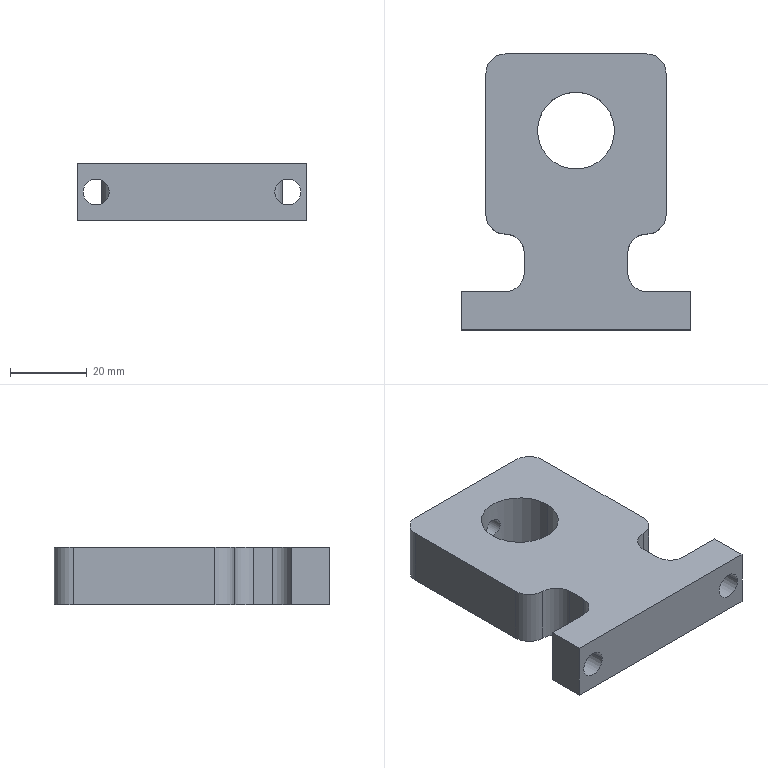Part | SolidWorks | features ICE 3, CirPattern 1, Extrusion 1, Fillet 1, HoleWzd 1 | 1 solid | 28 faces | box 60 x 72 x 15 mm | volume 42527 mm3 | cylinder 16 | plane 12 | commonest cylinder face diameters 10 x8 6.8 x4 5 x2 20.1 x2
STEP:
#1=CARTESIAN_POINT('',(0.,62.05,-2.5));
#2=VERTEX_POINT('',#1);
#3=CARTESIAN_POINT('',(0.,62.05,2.5));
#4=VERTEX_POINT('',#3);
#5=CARTESIAN_POINT('',(0.,62.05,-2.5));
#6=CARTESIAN_POINT('',(-0.327,62.05,-2.5));
#7=CARTESIAN_POINT('',(-0.6572,62.033,-2.434));
#8=CARTESIAN_POINT('',(-1.109,61.99,-2.247));
#9=CARTESIAN_POINT('',(-1.255,61.972,-2.168));
#10=CARTESIAN_POINT('',(-1.526,61.934,-1.987));
#11=CARTESIAN_POINT('',(-1.652,61.914,-1.884));
#12=CARTESIAN_POINT('',(-1.882,61.873,-1.653));
#13=CARTESIAN_POINT('',(-1.987,61.852,-1.525));
#14=CARTESIAN_POINT('',(-2.168,61.814,-1.255));
#15=CARTESIAN_POINT('',(-2.245,61.796,-1.112));
#16=CARTESIAN_POINT('',(-2.372,61.766,-0.808));
#17=CARTESIAN_POINT('',(-2.419,61.755,-0.6506));
#18=CARTESIAN_POINT('',(-2.483,61.738,-0.3307));
#19=CARTESIAN_POINT('',(-2.5,61.734,-0.1657));
#20=CARTESIAN_POINT('',(-2.5,61.734,0.1641));
#21=CARTESIAN_POINT('',(-2.484,61.738,0.3268));
#22=CARTESIAN_POINT('',(-2.42,61.754,0.6479));
#23=CARTESIAN_POINT('',(-2.372,61.766,0.8074));
#24=CARTESIAN_POINT('',(-2.247,61.796,1.109));
#25=CARTESIAN_POINT('',(-2.17,61.813,1.252));
#26=CARTESIAN_POINT('',(-1.988,61.852,1.525));
#27=CARTESIAN_POINT('',(-1.883,61.873,1.652));
#28=CARTESIAN_POINT('',(-1.654,61.914,1.882));
#29=CARTESIAN_POINT('',(-1.527,61.934,1.986));
#30=CARTESIAN_POINT('',(-1.255,61.972,2.168));
#31=CARTESIAN_POINT('',(-1.112,61.989,2.245));
#32=CARTESIAN_POINT('',(-0.8107,62.018,2.371));
#33=CARTESIAN_POINT('',(-0.6515,62.03,2.419));
#34=CARTESIAN_POINT('',(-0.3293,62.046,2.484));
#35=CARTESIAN_POINT('',(-0.1658,62.05,2.5));
#36=CARTESIAN_POINT('',(0.,62.05,2.5));
#37=B_SPLINE_CURVE_WITH_KNOTS('',3,(#5,#6,#7,#8,#9,#10,#11,#12,#13,#14,#15,#16,#17,#18,#19,#20,#21,#22,#23,#24,#25,#26,#27,#28,#29,#30,#31,#32,#33,#34,#35,#36),.UNSPECIFIED.,.F.,.F.,(4,2,2,2,2,2,2,2,2,2,2,2,2,2,2,4),(0.007847,0.008828,0.009318,0.009808,0.0103,0.01079,0.01128,0.01177,0.01226,0.01275,0.01324,0.01373,0.01422,0.01471,0.0152,0.01569),.UNSPECIFIED.);
#38=EDGE_CURVE('',#2,#4,#37,.T.);
#39=ORIENTED_EDGE('',*,*,#38,.F.);
#40=CARTESIAN_POINT('',(0.,72.,-2.5));
#41=VERTEX_POINT('',#40);
#42=CARTESIAN_POINT('',(0.,72.,-2.5));
#43=DIRECTION('',(0.,1.,0.));
#44=VECTOR('',#43,1000.);
#45=LINE('',#42,#44);
#46=EDGE_CURVE('',#2,#41,#45,.T.);
#47=ORIENTED_EDGE('',*,*,#46,.T.);
#48=CARTESIAN_POINT('',(0.,72.,2.5));
#49=VERTEX_POINT('',#48);
#50=CARTESIAN_POINT('',(0.,72.,0.));
#51=DIRECTION('',(0.,1.,0.));
#52=DIRECTION('',(0.,0.,1.));
#53=AXIS2_PLACEMENT_3D('',#50,#51,#52);
#54=CIRCLE('',#53,2.5);
#55=EDGE_CURVE('',#41,#49,#54,.T.);
#56=ORIENTED_EDGE('',*,*,#55,.T.);
#57=CARTESIAN_POINT('',(0.,72.,2.5));
#58=DIRECTION('',(0.,1.,0.));
#59=VECTOR('',#58,1000.);
#60=LINE('',#57,#59);
#61=EDGE_CURVE('',#4,#49,#60,.T.);
#62=ORIENTED_EDGE('',*,*,#61,.F.);
#63=EDGE_LOOP('',(#39,#47,#56,#62));
#64=FACE_OUTER_BOUND('',#63,.T.);
#65=CARTESIAN_POINT('',(0.,72.,0.));
#66=DIRECTION('',(0.,1.,0.));
#67=DIRECTION('',(0.,0.,1.));
#68=AXIS2_PLACEMENT_3D('',#65,#66,#67);
#69=CYLINDRICAL_SURFACE('',#68,2.5);
#70=ADVANCED_FACE('',(#64),#69,.F.);
#71=CARTESIAN_POINT('',(-21.6,10.,0.));
#72=VERTEX_POINT('',#71);
#73=CARTESIAN_POINT('',(-28.4,10.,0.));
#74=VERTEX_POINT('',#73);
#75=CARTESIAN_POINT('',(-25.,10.,0.));
#76=DIRECTION('',(0.,1.,0.));
#77=DIRECTION('',(1.,0.,0.));
#78=AXIS2_PLACEMENT_3D('',#75,#76,#77);
#79=CIRCLE('',#78,3.4);
#80=EDGE_CURVE('',#72,#74,#79,.T.);
#81=ORIENTED_EDGE('',*,*,#80,.T.);
#82=CARTESIAN_POINT('',(-28.4,0.,0.));
#83=VERTEX_POINT('',#82);
#84=CARTESIAN_POINT('',(-28.4,72.001,0.));
#85=DIRECTION('',(0.,-1.,0.));
#86=VECTOR('',#85,1000.);
#87=LINE('',#84,#86);
#88=EDGE_CURVE('',#74,#83,#87,.T.);
#89=ORIENTED_EDGE('',*,*,#88,.T.);
#90=CARTESIAN_POINT('',(-21.6,0.,0.));
#91=VERTEX_POINT('',#90);
#92=CARTESIAN_POINT('',(-25.,0.,0.));
#93=DIRECTION('',(0.,-1.,0.));
#94=DIRECTION('',(1.,0.,0.));
#95=AXIS2_PLACEMENT_3D('',#92,#93,#94);
#96=CIRCLE('',#95,3.4);
#97=EDGE_CURVE('',#83,#91,#96,.T.);
#98=ORIENTED_EDGE('',*,*,#97,.T.);
#99=CARTESIAN_POINT('',(-21.6,72.001,0.));
#100=DIRECTION('',(0.,-1.,0.));
#101=VECTOR('',#100,1000.);
#102=LINE('',#99,#101);
#103=EDGE_CURVE('',#72,#91,#102,.T.);
#104=ORIENTED_EDGE('',*,*,#103,.F.);
#105=EDGE_LOOP('',(#81,#89,#98,#104));
#106=FACE_OUTER_BOUND('',#105,.T.);
#107=CARTESIAN_POINT('',(-25.,72.001,0.));
#108=DIRECTION('',(0.,-1.,0.));
#109=DIRECTION('',(1.,0.,0.));
#110=AXIS2_PLACEMENT_3D('',#107,#108,#109);
#111=CYLINDRICAL_SURFACE('',#110,3.4);
#112=ADVANCED_FACE('',(#106),#111,.F.);
#113=CARTESIAN_POINT('',(28.4,10.,0.));
#114=VERTEX_POINT('',#113);
#115=CARTESIAN_POINT('',(21.6,10.,0.));
#116=VERTEX_POINT('',#115);
#117=CARTESIAN_POINT('',(25.,10.,0.));
#118=DIRECTION('',(0.,1.,0.));
#119=DIRECTION('',(1.,0.,0.));
#120=AXIS2_PLACEMENT_3D('',#117,#118,#119);
#121=CIRCLE('',#120,3.4);
#122=EDGE_CURVE('',#114,#116,#121,.T.);
#123=ORIENTED_EDGE('',*,*,#122,.T.);
#124=CARTESIAN_POINT('',(21.6,0.,0.));
#125=VERTEX_POINT('',#124);
#126=CARTESIAN_POINT('',(21.6,72.001,0.));
#127=DIRECTION('',(0.,-1.,0.));
#128=VECTOR('',#127,1000.);
#129=LINE('',#126,#128);
#130=EDGE_CURVE('',#116,#125,#129,.T.);
#131=ORIENTED_EDGE('',*,*,#130,.T.);
#132=CARTESIAN_POINT('',(28.4,0.,0.));
#133=VERTEX_POINT('',#132);
#134=CARTESIAN_POINT('',(25.,0.,0.));
#135=DIRECTION('',(0.,-1.,0.));
#136=DIRECTION('',(-1.,0.,0.));
#137=AXIS2_PLACEMENT_3D('',#134,#135,#136);
#138=CIRCLE('',#137,3.4);
#139=EDGE_CURVE('',#125,#133,#138,.T.);
#140=ORIENTED_EDGE('',*,*,#139,.T.);
#141=CARTESIAN_POINT('',(28.4,72.001,0.));
#142=DIRECTION('',(0.,-1.,0.));
#143=VECTOR('',#142,1000.);
#144=LINE('',#141,#143);
#145=EDGE_CURVE('',#114,#133,#144,.T.);
#146=ORIENTED_EDGE('',*,*,#145,.F.);
#147=EDGE_LOOP('',(#123,#131,#140,#146));
#148=FACE_OUTER_BOUND('',#147,.T.);
#149=CARTESIAN_POINT('',(25.,72.001,0.));
#150=DIRECTION('',(0.,-1.,0.));
#151=DIRECTION('',(1.,0.,0.));
#152=AXIS2_PLACEMENT_3D('',#149,#150,#151);
#153=CYLINDRICAL_SURFACE('',#152,3.4);
#154=ADVANCED_FACE('',(#148),#153,.F.);
#155=CARTESIAN_POINT('',(-10.05,52.,-7.5));
#156=VERTEX_POINT('',#155);
#157=CARTESIAN_POINT('',(10.05,52.,-7.5));
#158=VERTEX_POINT('',#157);
#159=CARTESIAN_POINT('',(0.,52.,-7.5));
#160=DIRECTION('',(0.,0.,1.));
#161=DIRECTION('',(1.,0.,0.));
#162=AXIS2_PLACEMENT_3D('',#159,#160,#161);
#163=CIRCLE('',#162,10.05);
#164=EDGE_CURVE('',#156,#158,#163,.T.);
#165=ORIENTED_EDGE('',*,*,#164,.F.);
#166=CARTESIAN_POINT('',(-10.05,52.,7.5));
#167=VERTEX_POINT('',#166);
#168=CARTESIAN_POINT('',(-10.05,52.,-7.5));
#169=DIRECTION('',(0.,0.,1.));
#170=VECTOR('',#169,1000.);
#171=LINE('',#168,#170);
#172=EDGE_CURVE('',#156,#167,#171,.T.);
#173=ORIENTED_EDGE('',*,*,#172,.T.);
#174=CARTESIAN_POINT('',(10.05,52.,7.5));
#175=VERTEX_POINT('',#174);
#176=CARTESIAN_POINT('',(0.,52.,7.5));
#177=DIRECTION('',(0.,0.,1.));
#178=DIRECTION('',(1.,0.,0.));
#179=AXIS2_PLACEMENT_3D('',#176,#177,#178);
#180=CIRCLE('',#179,10.05);
#181=EDGE_CURVE('',#167,#175,#180,.T.);
#182=ORIENTED_EDGE('',*,*,#181,.T.);
#183=CARTESIAN_POINT('',(10.05,52.,-7.5));
#184=DIRECTION('',(0.,0.,1.));
#185=VECTOR('',#184,1000.);
#186=LINE('',#183,#185);
#187=EDGE_CURVE('',#158,#175,#186,.T.);
#188=ORIENTED_EDGE('',*,*,#187,.F.);
#189=EDGE_LOOP('',(#165,#173,#182,#188));
#190=FACE_OUTER_BOUND('',#189,.T.);
#191=CARTESIAN_POINT('',(0.,52.,-7.5));
#192=DIRECTION('',(0.,0.,1.));
#193=DIRECTION('',(1.,0.,0.));
#194=AXIS2_PLACEMENT_3D('',#191,#192,#193);
#195=CYLINDRICAL_SURFACE('',#194,10.05);
#196=ADVANCED_FACE('',(#190),#195,.F.);
#197=CARTESIAN_POINT('',(23.5,30.,-7.5));
#198=VERTEX_POINT('',#197);
#199=CARTESIAN_POINT('',(23.5,67.,-7.5));
#200=VERTEX_POINT('',#199);
#201=CARTESIAN_POINT('',(23.5,25.,-7.5));
#202=DIRECTION('',(0.,1.,0.));
#203=VECTOR('',#202,1000.);
#204=LINE('',#201,#203);
#205=EDGE_CURVE('',#198,#200,#204,.T.);
#206=ORIENTED_EDGE('',*,*,#205,.T.);
#207=CARTESIAN_POINT('',(23.5,67.,7.5));
#208=VERTEX_POINT('',#207);
#209=CARTESIAN_POINT('',(23.5,67.,7.5));
#210=DIRECTION('',(0.,0.,1.));
#211=VECTOR('',#210,1000.);
#212=LINE('',#209,#211);
#213=EDGE_CURVE('',#200,#208,#212,.T.);
#214=ORIENTED_EDGE('',*,*,#213,.T.);
#215=CARTESIAN_POINT('',(23.5,30.,7.5));
#216=VERTEX_POINT('',#215);
#217=CARTESIAN_POINT('',(23.5,25.,7.5));
#218=DIRECTION('',(0.,1.,0.));
#219=VECTOR('',#218,1000.);
#220=LINE('',#217,#219);
#221=EDGE_CURVE('',#216,#208,#220,.T.);
#222=ORIENTED_EDGE('',*,*,#221,.F.);
#223=CARTESIAN_POINT('',(23.5,30.,7.5));
#224=DIRECTION('',(0.,0.,-1.));
#225=VECTOR('',#224,1000.);
#226=LINE('',#223,#225);
#227=EDGE_CURVE('',#216,#198,#226,.T.);
#228=ORIENTED_EDGE('',*,*,#227,.T.);
#229=EDGE_LOOP('',(#206,#214,#222,#228));
#230=FACE_OUTER_BOUND('',#229,.T.);
#231=CARTESIAN_POINT('',(23.5,25.,7.5));
#232=DIRECTION('',(-1.,0.,0.));
#233=DIRECTION('',(0.,-1.,0.));
#234=AXIS2_PLACEMENT_3D('',#231,#232,#233);
#235=PLANE('',#234);
#236=ADVANCED_FACE('',(#230),#235,.F.);
#237=CARTESIAN_POINT('',(0.,72.,0.));
#238=DIRECTION('',(0.,1.,0.));
#239=DIRECTION('',(0.,0.,1.));
#240=AXIS2_PLACEMENT_3D('',#237,#238,#239);
#241=CIRCLE('',#240,2.5);
#242=EDGE_CURVE('',#49,#41,#241,.T.);
#243=ORIENTED_EDGE('',*,*,#242,.F.);
#244=ORIENTED_EDGE('',*,*,#55,.F.);
#245=EDGE_LOOP('',(#243,#244));
#246=FACE_BOUND('',#245,.T.);
#247=CARTESIAN_POINT('',(18.5,72.,7.5));
#248=VERTEX_POINT('',#247);
#249=CARTESIAN_POINT('',(-18.5,72.,7.5));
#250=VERTEX_POINT('',#249);
#251=CARTESIAN_POINT('',(-23.5,72.,7.5));
#252=DIRECTION('',(-1.,0.,0.));
#253=VECTOR('',#252,1000.);
#254=LINE('',#251,#253);
#255=EDGE_CURVE('',#248,#250,#254,.T.);
#256=ORIENTED_EDGE('',*,*,#255,.F.);
#257=CARTESIAN_POINT('',(18.5,72.,-7.5));
#258=VERTEX_POINT('',#257);
#259=CARTESIAN_POINT('',(18.5,72.,7.5));
#260=DIRECTION('',(0.,0.,-1.));
#261=VECTOR('',#260,1000.);
#262=LINE('',#259,#261);
#263=EDGE_CURVE('',#248,#258,#262,.T.);
#264=ORIENTED_EDGE('',*,*,#263,.T.);
#265=CARTESIAN_POINT('',(-18.5,72.,-7.5));
#266=VERTEX_POINT('',#265);
#267=CARTESIAN_POINT('',(-23.5,72.,-7.5));
#268=DIRECTION('',(-1.,0.,0.));
#269=VECTOR('',#268,1000.);
#270=LINE('',#267,#269);
#271=EDGE_CURVE('',#258,#266,#270,.T.);
#272=ORIENTED_EDGE('',*,*,#271,.T.);
#273=CARTESIAN_POINT('',(-18.5,72.,7.5));
#274=DIRECTION('',(0.,0.,1.));
#275=VECTOR('',#274,1000.);
#276=LINE('',#273,#275);
#277=EDGE_CURVE('',#266,#250,#276,.T.);
#278=ORIENTED_EDGE('',*,*,#277,.T.);
#279=EDGE_LOOP('',(#256,#264,#272,#278));
#280=FACE_OUTER_BOUND('',#279,.T.);
#281=CARTESIAN_POINT('',(-23.5,72.,7.5));
#282=DIRECTION('',(0.,-1.,0.));
#283=DIRECTION('',(0.,0.,-1.));
#284=AXIS2_PLACEMENT_3D('',#281,#282,#283);
#285=PLANE('',#284);
#286=ADVANCED_FACE('',(#246,#280),#285,.F.);
#287=CARTESIAN_POINT('',(-23.5,67.,7.5));
#288=VERTEX_POINT('',#287);
#289=CARTESIAN_POINT('',(-23.5,30.,7.5));
#290=VERTEX_POINT('',#289);
#291=CARTESIAN_POINT('',(-23.5,25.,7.5));
#292=DIRECTION('',(0.,-1.,0.));
#293=VECTOR('',#292,1000.);
#294=LINE('',#291,#293);
#295=EDGE_CURVE('',#288,#290,#294,.T.);
#296=ORIENTED_EDGE('',*,*,#295,.F.);
#297=CARTESIAN_POINT('',(-23.5,67.,-7.5));
#298=VERTEX_POINT('',#297);
#299=CARTESIAN_POINT('',(-23.5,67.,7.5));
#300=DIRECTION('',(0.,0.,-1.));
#301=VECTOR('',#300,1000.);
#302=LINE('',#299,#301);
#303=EDGE_CURVE('',#288,#298,#302,.T.);
#304=ORIENTED_EDGE('',*,*,#303,.T.);
#305=CARTESIAN_POINT('',(-23.5,30.,-7.5));
#306=VERTEX_POINT('',#305);
#307=CARTESIAN_POINT('',(-23.5,25.,-7.5));
#308=DIRECTION('',(0.,-1.,0.));
#309=VECTOR('',#308,1000.);
#310=LINE('',#307,#309);
#311=EDGE_CURVE('',#298,#306,#310,.T.);
#312=ORIENTED_EDGE('',*,*,#311,.T.);
#313=CARTESIAN_POINT('',(-23.5,30.,7.5));
#314=DIRECTION('',(0.,0.,1.));
#315=VECTOR('',#314,1000.);
#316=LINE('',#313,#315);
#317=EDGE_CURVE('',#306,#290,#316,.T.);
#318=ORIENTED_EDGE('',*,*,#317,.T.);
#319=EDGE_LOOP('',(#296,#304,#312,#318));
#320=FACE_OUTER_BOUND('',#319,.T.);
#321=CARTESIAN_POINT('',(-23.5,25.,7.5));
#322=DIRECTION('',(1.,0.,0.));
#323=DIRECTION('',(0.,1.,0.));
#324=AXIS2_PLACEMENT_3D('',#321,#322,#323);
#325=PLANE('',#324);
#326=ADVANCED_FACE('',(#320),#325,.F.);
#327=CARTESIAN_POINT('',(-13.5,20.,-7.5));
#328=VERTEX_POINT('',#327);
#329=CARTESIAN_POINT('',(-13.5,15.,-7.5));
#330=VERTEX_POINT('',#329);
#331=CARTESIAN_POINT('',(-13.5,10.,-7.5));
#332=DIRECTION('',(0.,-1.,0.));
#333=VECTOR('',#332,1000.);
#334=LINE('',#331,#333);
#335=EDGE_CURVE('',#328,#330,#334,.T.);
#336=ORIENTED_EDGE('',*,*,#335,.T.);
#337=CARTESIAN_POINT('',(-13.5,15.,7.5));
#338=VERTEX_POINT('',#337);
#339=CARTESIAN_POINT('',(-13.5,15.,7.5));
#340=DIRECTION('',(0.,0.,1.));
#341=VECTOR('',#340,1000.);
#342=LINE('',#339,#341);
#343=EDGE_CURVE('',#330,#338,#342,.T.);
#344=ORIENTED_EDGE('',*,*,#343,.T.);
#345=CARTESIAN_POINT('',(-13.5,20.,7.5));
#346=VERTEX_POINT('',#345);
#347=CARTESIAN_POINT('',(-13.5,10.,7.5));
#348=DIRECTION('',(0.,-1.,0.));
#349=VECTOR('',#348,1000.);
#350=LINE('',#347,#349);
#351=EDGE_CURVE('',#346,#338,#350,.T.);
#352=ORIENTED_EDGE('',*,*,#351,.F.);
#353=CARTESIAN_POINT('',(-13.5,20.,-7.5));
#354=DIRECTION('',(0.,0.,-1.));
#355=VECTOR('',#354,1000.);
#356=LINE('',#353,#355);
#357=EDGE_CURVE('',#346,#328,#356,.T.);
#358=ORIENTED_EDGE('',*,*,#357,.T.);
#359=EDGE_LOOP('',(#336,#344,#352,#358));
#360=FACE_OUTER_BOUND('',#359,.T.);
#361=CARTESIAN_POINT('',(-13.5,10.,7.5));
#362=DIRECTION('',(1.,0.,0.));
#363=DIRECTION('',(0.,1.,0.));
#364=AXIS2_PLACEMENT_3D('',#361,#362,#363);
#365=PLANE('',#364);
#366=ADVANCED_FACE('',(#360),#365,.F.);
#367=ORIENTED_EDGE('',*,*,#80,.F.);
#368=CARTESIAN_POINT('',(-25.,10.,0.));
#369=DIRECTION('',(0.,1.,0.));
#370=DIRECTION('',(1.,0.,0.));
#371=AXIS2_PLACEMENT_3D('',#368,#369,#370);
#372=CIRCLE('',#371,3.4);
#373=EDGE_CURVE('',#74,#72,#372,.T.);
#374=ORIENTED_EDGE('',*,*,#373,.F.);
#375=EDGE_LOOP('',(#367,#374));
#376=FACE_BOUND('',#375,.T.);
#377=CARTESIAN_POINT('',(-18.5,10.,7.5));
#378=VERTEX_POINT('',#377);
#379=CARTESIAN_POINT('',(-30.,10.,7.5));
#380=VERTEX_POINT('',#379);
#381=CARTESIAN_POINT('',(-30.,10.,7.5));
#382=DIRECTION('',(-1.,0.,0.));
#383=VECTOR('',#382,1000.);
#384=LINE('',#381,#383);
#385=EDGE_CURVE('',#378,#380,#384,.T.);
#386=ORIENTED_EDGE('',*,*,#385,.F.);
#387=CARTESIAN_POINT('',(-18.5,10.,-7.5));
#388=VERTEX_POINT('',#387);
#389=CARTESIAN_POINT('',(-18.5,10.,-7.5));
#390=DIRECTION('',(0.,0.,-1.));
#391=VECTOR('',#390,1000.);
#392=LINE('',#389,#391);
#393=EDGE_CURVE('',#378,#388,#392,.T.);
#394=ORIENTED_EDGE('',*,*,#393,.T.);
#395=CARTESIAN_POINT('',(-30.,10.,-7.5));
#396=VERTEX_POINT('',#395);
#397=CARTESIAN_POINT('',(-30.,10.,-7.5));
#398=DIRECTION('',(-1.,0.,0.));
#399=VECTOR('',#398,1000.);
#400=LINE('',#397,#399);
#401=EDGE_CURVE('',#388,#396,#400,.T.);
#402=ORIENTED_EDGE('',*,*,#401,.T.);
#403=CARTESIAN_POINT('',(-30.,10.,7.5));
#404=DIRECTION('',(0.,0.,-1.));
#405=VECTOR('',#404,1000.);
#406=LINE('',#403,#405);
#407=EDGE_CURVE('',#380,#396,#406,.T.);
#408=ORIENTED_EDGE('',*,*,#407,.F.);
#409=EDGE_LOOP('',(#386,#394,#402,#408));
#410=FACE_OUTER_BOUND('',#409,.T.);
#411=CARTESIAN_POINT('',(-30.,10.,7.5));
#412=DIRECTION('',(0.,-1.,0.));
#413=DIRECTION('',(1.,0.,0.));
#414=AXIS2_PLACEMENT_3D('',#411,#412,#413);
#415=PLANE('',#414);
#416=ADVANCED_FACE('',(#376,#410),#415,.F.);
#417=CARTESIAN_POINT('',(-30.,0.,-7.5));
#418=VERTEX_POINT('',#417);
#419=CARTESIAN_POINT('',(-30.,0.,-7.5));
#420=DIRECTION('',(0.,-1.,0.));
#421=VECTOR('',#420,1000.);
#422=LINE('',#419,#421);
#423=EDGE_CURVE('',#396,#418,#422,.T.);
#424=ORIENTED_EDGE('',*,*,#423,.T.);
#425=CARTESIAN_POINT('',(-30.,0.,7.5));
#426=VERTEX_POINT('',#425);
#427=CARTESIAN_POINT('',(-30.,0.,7.5));
#428=DIRECTION('',(0.,0.,-1.));
#429=VECTOR('',#428,1000.);
#430=LINE('',#427,#429);
#431=EDGE_CURVE('',#426,#418,#430,.T.);
#432=ORIENTED_EDGE('',*,*,#431,.F.);
#433=CARTESIAN_POINT('',(-30.,0.,7.5));
#434=DIRECTION('',(0.,-1.,0.));
#435=VECTOR('',#434,1000.);
#436=LINE('',#433,#435);
#437=EDGE_CURVE('',#380,#426,#436,.T.);
#438=ORIENTED_EDGE('',*,*,#437,.F.);
#439=ORIENTED_EDGE('',*,*,#407,.T.);
#440=EDGE_LOOP('',(#424,#432,#438,#439));
#441=FACE_OUTER_BOUND('',#440,.T.);
#442=CARTESIAN_POINT('',(-30.,0.,7.5));
#443=DIRECTION('',(1.,0.,0.));
#444=DIRECTION('',(0.,0.,-1.));
#445=AXIS2_PLACEMENT_3D('',#442,#443,#444);
#446=PLANE('',#445);
#447=ADVANCED_FACE('',(#441),#446,.F.);
#448=CARTESIAN_POINT('',(-25.,0.,0.));
#449=DIRECTION('',(0.,-1.,0.));
#450=DIRECTION('',(1.,0.,0.));
#451=AXIS2_PLACEMENT_3D('',#448,#449,#450);
#452=CIRCLE('',#451,3.4);
#453=EDGE_CURVE('',#91,#83,#452,.T.);
#454=ORIENTED_EDGE('',*,*,#453,.F.);
#455=ORIENTED_EDGE('',*,*,#97,.F.);
#456=EDGE_LOOP('',(#454,#455));
#457=FACE_BOUND('',#456,.T.);
#458=CARTESIAN_POINT('',(25.,0.,0.));
#459=DIRECTION('',(0.,-1.,0.));
#460=DIRECTION('',(-1.,0.,0.));
#461=AXIS2_PLACEMENT_3D('',#458,#459,#460);
#462=CIRCLE('',#461,3.4);
#463=EDGE_CURVE('',#133,#125,#462,.T.);
#464=ORIENTED_EDGE('',*,*,#463,.F.);
#465=ORIENTED_EDGE('',*,*,#139,.F.);
#466=EDGE_LOOP('',(#464,#465));
#467=FACE_BOUND('',#466,.T.);
#468=CARTESIAN_POINT('',(30.,0.,-7.5));
#469=VERTEX_POINT('',#468);
#470=CARTESIAN_POINT('',(30.,0.,-7.5));
#471=DIRECTION('',(1.,0.,0.));
#472=VECTOR('',#471,1000.);
#473=LINE('',#470,#472);
#474=EDGE_CURVE('',#418,#469,#473,.T.);
#475=ORIENTED_EDGE('',*,*,#474,.T.);
#476=CARTESIAN_POINT('',(30.,0.,7.5));
#477=VERTEX_POINT('',#476);
#478=CARTESIAN_POINT('',(30.,0.,7.5));
#479=DIRECTION('',(0.,0.,-1.));
#480=VECTOR('',#479,1000.);
#481=LINE('',#478,#480);
#482=EDGE_CURVE('',#477,#469,#481,.T.);
#483=ORIENTED_EDGE('',*,*,#482,.F.);
#484=CARTESIAN_POINT('',(30.,0.,7.5));
#485=DIRECTION('',(1.,0.,0.));
#486=VECTOR('',#485,1000.);
#487=LINE('',#484,#486);
#488=EDGE_CURVE('',#426,#477,#487,.T.);
#489=ORIENTED_EDGE('',*,*,#488,.F.);
#490=ORIENTED_EDGE('',*,*,#431,.T.);
#491=EDGE_LOOP('',(#475,#483,#489,#490));
#492=FACE_OUTER_BOUND('',#491,.T.);
#493=CARTESIAN_POINT('',(30.,0.,7.5));
#494=DIRECTION('',(0.,1.,0.));
#495=DIRECTION('',(-1.,0.,0.));
#496=AXIS2_PLACEMENT_3D('',#493,#494,#495);
#497=PLANE('',#496);
#498=ADVANCED_FACE('',(#457,#467,#492),#497,.F.);
#499=CARTESIAN_POINT('',(30.,10.,-7.5));
#500=VERTEX_POINT('',#499);
#501=CARTESIAN_POINT('',(30.,0.,-7.5));
#502=DIRECTION('',(0.,1.,0.));
#503=VECTOR('',#502,1000.);
#504=LINE('',#501,#503);
#505=EDGE_CURVE('',#469,#500,#504,.T.);
#506=ORIENTED_EDGE('',*,*,#505,.T.);
#507=CARTESIAN_POINT('',(30.,10.,7.5));
#508=VERTEX_POINT('',#507);
#509=CARTESIAN_POINT('',(30.,10.,7.5));
#510=DIRECTION('',(0.,0.,-1.));
#511=VECTOR('',#510,1000.);
#512=LINE('',#509,#511);
#513=EDGE_CURVE('',#508,#500,#512,.T.);
#514=ORIENTED_EDGE('',*,*,#513,.F.);
#515=CARTESIAN_POINT('',(30.,0.,7.5));
#516=DIRECTION('',(0.,1.,0.));
#517=VECTOR('',#516,1000.);
#518=LINE('',#515,#517);
#519=EDGE_CURVE('',#477,#508,#518,.T.);
#520=ORIENTED_EDGE('',*,*,#519,.F.);
#521=ORIENTED_EDGE('',*,*,#482,.T.);
#522=EDGE_LOOP('',(#506,#514,#520,#521));
#523=FACE_OUTER_BOUND('',#522,.T.);
#524=CARTESIAN_POINT('',(30.,0.,7.5));
#525=DIRECTION('',(-1.,0.,0.));
#526=DIRECTION('',(0.,-1.,0.));
#527=AXIS2_PLACEMENT_3D('',#524,#525,#526);
#528=PLANE('',#527);
#529=ADVANCED_FACE('',(#523),#528,.F.);
#530=ORIENTED_EDGE('',*,*,#122,.F.);
#531=CARTESIAN_POINT('',(25.,10.,0.));
#532=DIRECTION('',(0.,1.,0.));
#533=DIRECTION('',(1.,0.,0.));
#534=AXIS2_PLACEMENT_3D('',#531,#532,#533);
#535=CIRCLE('',#534,3.4);
#536=EDGE_CURVE('',#116,#114,#535,.T.);
#537=ORIENTED_EDGE('',*,*,#536,.F.);
#538=EDGE_LOOP('',(#530,#537));
#539=FACE_BOUND('',#538,.T.);
#540=CARTESIAN_POINT('',(18.5,10.,-7.5));
#541=VERTEX_POINT('',#540);
#542=CARTESIAN_POINT('',(30.,10.,-7.5));
#543=DIRECTION('',(-1.,0.,0.));
#544=VECTOR('',#543,1000.);
#545=LINE('',#542,#544);
#546=EDGE_CURVE('',#500,#541,#545,.T.);
#547=ORIENTED_EDGE('',*,*,#546,.T.);
#548=CARTESIAN_POINT('',(18.5,10.,7.5));
#549=VERTEX_POINT('',#548);
#550=CARTESIAN_POINT('',(18.5,10.,7.5));
#551=DIRECTION('',(0.,0.,1.));
#552=VECTOR('',#551,1000.);
#553=LINE('',#550,#552);
#554=EDGE_CURVE('',#541,#549,#553,.T.);
#555=ORIENTED_EDGE('',*,*,#554,.T.);
#556=CARTESIAN_POINT('',(30.,10.,7.5));
#557=DIRECTION('',(-1.,0.,0.));
#558=VECTOR('',#557,1000.);
#559=LINE('',#556,#558);
#560=EDGE_CURVE('',#508,#549,#559,.T.);
#561=ORIENTED_EDGE('',*,*,#560,.F.);
#562=ORIENTED_EDGE('',*,*,#513,.T.);
#563=EDGE_LOOP('',(#547,#555,#561,#562));
#564=FACE_OUTER_BOUND('',#563,.T.);
#565=CARTESIAN_POINT('',(30.,10.,7.5));
#566=DIRECTION('',(0.,-1.,0.));
#567=DIRECTION('',(1.,0.,0.));
#568=AXIS2_PLACEMENT_3D('',#565,#566,#567);
#569=PLANE('',#568);
#570=ADVANCED_FACE('',(#539,#564),#569,.F.);
#571=CARTESIAN_POINT('',(13.5,15.,7.5));
#572=VERTEX_POINT('',#571);
#573=CARTESIAN_POINT('',(13.5,20.,7.5));
#574=VERTEX_POINT('',#573);
#575=CARTESIAN_POINT('',(13.5,10.,7.5));
#576=DIRECTION('',(0.,1.,0.));
#577=VECTOR('',#576,1000.);
#578=LINE('',#575,#577);
#579=EDGE_CURVE('',#572,#574,#578,.T.);
#580=ORIENTED_EDGE('',*,*,#579,.F.);
#581=CARTESIAN_POINT('',(13.5,15.,-7.5));
#582=VERTEX_POINT('',#581);
#583=CARTESIAN_POINT('',(13.5,15.,-7.5));
#584=DIRECTION('',(0.,0.,-1.));
#585=VECTOR('',#584,1000.);
#586=LINE('',#583,#585);
#587=EDGE_CURVE('',#572,#582,#586,.T.);
#588=ORIENTED_EDGE('',*,*,#587,.T.);
#589=CARTESIAN_POINT('',(13.5,20.,-7.5));
#590=VERTEX_POINT('',#589);
#591=CARTESIAN_POINT('',(13.5,10.,-7.5));
#592=DIRECTION('',(0.,1.,0.));
#593=VECTOR('',#592,1000.);
#594=LINE('',#591,#593);
#595=EDGE_CURVE('',#582,#590,#594,.T.);
#596=ORIENTED_EDGE('',*,*,#595,.T.);
#597=CARTESIAN_POINT('',(13.5,20.,7.5));
#598=DIRECTION('',(0.,0.,1.));
#599=VECTOR('',#598,1000.);
#600=LINE('',#597,#599);
#601=EDGE_CURVE('',#590,#574,#600,.T.);
#602=ORIENTED_EDGE('',*,*,#601,.T.);
#603=EDGE_LOOP('',(#580,#588,#596,#602));
#604=FACE_OUTER_BOUND('',#603,.T.);
#605=CARTESIAN_POINT('',(13.5,10.,7.5));
#606=DIRECTION('',(-1.,0.,0.));
#607=DIRECTION('',(0.,-1.,0.));
#608=AXIS2_PLACEMENT_3D('',#605,#606,#607);
#609=PLANE('',#608);
#610=ADVANCED_FACE('',(#604),#609,.F.);
#611=CARTESIAN_POINT('',(0.,52.,7.5));
#612=DIRECTION('',(0.,0.,1.));
#613=DIRECTION('',(1.,0.,0.));
#614=AXIS2_PLACEMENT_3D('',#611,#612,#613);
#615=CIRCLE('',#614,10.05);
#616=EDGE_CURVE('',#175,#167,#615,.T.);
#617=ORIENTED_EDGE('',*,*,#616,.F.);
#618=ORIENTED_EDGE('',*,*,#181,.F.);
#619=EDGE_LOOP('',(#617,#618));
#620=FACE_BOUND('',#619,.T.);
#621=ORIENTED_EDGE('',*,*,#221,.T.);
#622=CARTESIAN_POINT('',(18.5,67.,7.5));
#623=DIRECTION('',(0.,0.,1.));
#624=DIRECTION('',(-1.,0.,0.));
#625=AXIS2_PLACEMENT_3D('',#622,#623,#624);
#626=CIRCLE('',#625,5.);
#627=EDGE_CURVE('',#208,#248,#626,.T.);
#628=ORIENTED_EDGE('',*,*,#627,.T.);
#629=ORIENTED_EDGE('',*,*,#255,.T.);
#630=CARTESIAN_POINT('',(-18.5,67.,7.5));
#631=DIRECTION('',(0.,0.,1.));
#632=DIRECTION('',(-1.,0.,0.));
#633=AXIS2_PLACEMENT_3D('',#630,#631,#632);
#634=CIRCLE('',#633,5.);
#635=EDGE_CURVE('',#250,#288,#634,.T.);
#636=ORIENTED_EDGE('',*,*,#635,.T.);
#637=ORIENTED_EDGE('',*,*,#295,.T.);
#638=CARTESIAN_POINT('',(-18.5,25.,7.5));
#639=VERTEX_POINT('',#638);
#640=CARTESIAN_POINT('',(-18.5,30.,7.5));
#641=DIRECTION('',(0.,0.,1.));
#642=DIRECTION('',(-1.,0.,0.));
#643=AXIS2_PLACEMENT_3D('',#640,#641,#642);
#644=CIRCLE('',#643,5.);
#645=EDGE_CURVE('',#290,#639,#644,.T.);
#646=ORIENTED_EDGE('',*,*,#645,.T.);
#647=CARTESIAN_POINT('',(-18.5,20.,7.5));
#648=DIRECTION('',(0.,0.,-1.));
#649=DIRECTION('',(-1.,0.,0.));
#650=AXIS2_PLACEMENT_3D('',#647,#648,#649);
#651=CIRCLE('',#650,5.);
#652=EDGE_CURVE('',#639,#346,#651,.T.);
#653=ORIENTED_EDGE('',*,*,#652,.T.);
#654=ORIENTED_EDGE('',*,*,#351,.T.);
#655=CARTESIAN_POINT('',(-18.5,15.,7.5));
#656=DIRECTION('',(0.,0.,-1.));
#657=DIRECTION('',(-1.,0.,0.));
#658=AXIS2_PLACEMENT_3D('',#655,#656,#657);
#659=CIRCLE('',#658,5.);
#660=EDGE_CURVE('',#338,#378,#659,.T.);
#661=ORIENTED_EDGE('',*,*,#660,.T.);
#662=ORIENTED_EDGE('',*,*,#385,.T.);
#663=ORIENTED_EDGE('',*,*,#437,.T.);
#664=ORIENTED_EDGE('',*,*,#488,.T.);
#665=ORIENTED_EDGE('',*,*,#519,.T.);
#666=ORIENTED_EDGE('',*,*,#560,.T.);
#667=CARTESIAN_POINT('',(18.5,15.,7.5));
#668=DIRECTION('',(0.,0.,-1.));
#669=DIRECTION('',(-1.,0.,0.));
#670=AXIS2_PLACEMENT_3D('',#667,#668,#669);
#671=CIRCLE('',#670,5.);
#672=EDGE_CURVE('',#549,#572,#671,.T.);
#673=ORIENTED_EDGE('',*,*,#672,.T.);
#674=ORIENTED_EDGE('',*,*,#579,.T.);
#675=CARTESIAN_POINT('',(18.5,25.,7.5));
#676=VERTEX_POINT('',#675);
#677=CARTESIAN_POINT('',(18.5,20.,7.5));
#678=DIRECTION('',(0.,0.,-1.));
#679=DIRECTION('',(-1.,0.,0.));
#680=AXIS2_PLACEMENT_3D('',#677,#678,#679);
#681=CIRCLE('',#680,5.);
#682=EDGE_CURVE('',#574,#676,#681,.T.);
#683=ORIENTED_EDGE('',*,*,#682,.T.);
#684=CARTESIAN_POINT('',(18.5,30.,7.5));
#685=DIRECTION('',(0.,0.,1.));
#686=DIRECTION('',(-1.,0.,0.));
#687=AXIS2_PLACEMENT_3D('',#684,#685,#686);
#688=CIRCLE('',#687,5.);
#689=EDGE_CURVE('',#676,#216,#688,.T.);
#690=ORIENTED_EDGE('',*,*,#689,.T.);
#691=EDGE_LOOP('',(#621,#628,#629,#636,#637,#646,#653,#654,#661,#662,#663,#664,#665,#666,#673,#674,#683,#690));
#692=FACE_OUTER_BOUND('',#691,.T.);
#693=CARTESIAN_POINT('',(0.,0.,7.5));
#694=DIRECTION('',(0.,0.,-1.));
#695=DIRECTION('',(-1.,0.,0.));
#696=AXIS2_PLACEMENT_3D('',#693,#694,#695);
#697=PLANE('',#696);
#698=ADVANCED_FACE('',(#620,#692),#697,.F.);
#699=CARTESIAN_POINT('',(0.,52.,-7.5));
#700=DIRECTION('',(0.,0.,1.));
#701=DIRECTION('',(1.,0.,0.));
#702=AXIS2_PLACEMENT_3D('',#699,#700,#701);
#703=CIRCLE('',#702,10.05);
#704=EDGE_CURVE('',#158,#156,#703,.T.);
#705=ORIENTED_EDGE('',*,*,#704,.T.);
#706=ORIENTED_EDGE('',*,*,#164,.T.);
#707=EDGE_LOOP('',(#705,#706));
#708=FACE_BOUND('',#707,.T.);
#709=ORIENTED_EDGE('',*,*,#271,.F.);
#710=CARTESIAN_POINT('',(18.5,67.,-7.5));
#711=DIRECTION('',(0.,0.,-1.));
#712=DIRECTION('',(-1.,0.,0.));
#713=AXIS2_PLACEMENT_3D('',#710,#711,#712);
#714=CIRCLE('',#713,5.);
#715=EDGE_CURVE('',#258,#200,#714,.T.);
#716=ORIENTED_EDGE('',*,*,#715,.T.);
#717=ORIENTED_EDGE('',*,*,#205,.F.);
#718=CARTESIAN_POINT('',(18.5,25.,-7.5));
#719=VERTEX_POINT('',#718);
#720=CARTESIAN_POINT('',(18.5,30.,-7.5));
#721=DIRECTION('',(0.,0.,-1.));
#722=DIRECTION('',(-1.,0.,0.));
#723=AXIS2_PLACEMENT_3D('',#720,#721,#722);
#724=CIRCLE('',#723,5.);
#725=EDGE_CURVE('',#198,#719,#724,.T.);
#726=ORIENTED_EDGE('',*,*,#725,.T.);
#727=CARTESIAN_POINT('',(18.5,20.,-7.5));
#728=DIRECTION('',(0.,0.,1.));
#729=DIRECTION('',(-1.,0.,0.));
#730=AXIS2_PLACEMENT_3D('',#727,#728,#729);
#731=CIRCLE('',#730,5.);
#732=EDGE_CURVE('',#719,#590,#731,.T.);
#733=ORIENTED_EDGE('',*,*,#732,.T.);
#734=ORIENTED_EDGE('',*,*,#595,.F.);
#735=CARTESIAN_POINT('',(18.5,15.,-7.5));
#736=DIRECTION('',(0.,0.,1.));
#737=DIRECTION('',(-1.,0.,0.));
#738=AXIS2_PLACEMENT_3D('',#735,#736,#737);
#739=CIRCLE('',#738,5.);
#740=EDGE_CURVE('',#582,#541,#739,.T.);
#741=ORIENTED_EDGE('',*,*,#740,.T.);
#742=ORIENTED_EDGE('',*,*,#546,.F.);
#743=ORIENTED_EDGE('',*,*,#505,.F.);
#744=ORIENTED_EDGE('',*,*,#474,.F.);
#745=ORIENTED_EDGE('',*,*,#423,.F.);
#746=ORIENTED_EDGE('',*,*,#401,.F.);
#747=CARTESIAN_POINT('',(-18.5,15.,-7.5));
#748=DIRECTION('',(0.,0.,1.));
#749=DIRECTION('',(-1.,0.,0.));
#750=AXIS2_PLACEMENT_3D('',#747,#748,#749);
#751=CIRCLE('',#750,5.);
#752=EDGE_CURVE('',#388,#330,#751,.T.);
#753=ORIENTED_EDGE('',*,*,#752,.T.);
#754=ORIENTED_EDGE('',*,*,#335,.F.);
#755=CARTESIAN_POINT('',(-18.5,25.,-7.5));
#756=VERTEX_POINT('',#755);
#757=CARTESIAN_POINT('',(-18.5,20.,-7.5));
#758=DIRECTION('',(0.,0.,1.));
#759=DIRECTION('',(-1.,0.,0.));
#760=AXIS2_PLACEMENT_3D('',#757,#758,#759);
#761=CIRCLE('',#760,5.);
#762=EDGE_CURVE('',#328,#756,#761,.T.);
#763=ORIENTED_EDGE('',*,*,#762,.T.);
#764=CARTESIAN_POINT('',(-18.5,30.,-7.5));
#765=DIRECTION('',(0.,0.,-1.));
#766=DIRECTION('',(-1.,0.,0.));
#767=AXIS2_PLACEMENT_3D('',#764,#765,#766);
#768=CIRCLE('',#767,5.);
#769=EDGE_CURVE('',#756,#306,#768,.T.);
#770=ORIENTED_EDGE('',*,*,#769,.T.);
#771=ORIENTED_EDGE('',*,*,#311,.F.);
#772=CARTESIAN_POINT('',(-18.5,67.,-7.5));
#773=DIRECTION('',(0.,0.,-1.));
#774=DIRECTION('',(-1.,0.,0.));
#775=AXIS2_PLACEMENT_3D('',#772,#773,#774);
#776=CIRCLE('',#775,5.);
#777=EDGE_CURVE('',#298,#266,#776,.T.);
#778=ORIENTED_EDGE('',*,*,#777,.T.);
#779=EDGE_LOOP('',(#709,#716,#717,#726,#733,#734,#741,#742,#743,#744,#745,#746,#753,#754,#763,#770,#771,#778));
#780=FACE_OUTER_BOUND('',#779,.T.);
#781=CARTESIAN_POINT('',(0.,0.,-7.5));
#782=DIRECTION('',(0.,0.,-1.));
#783=DIRECTION('',(-1.,0.,0.));
#784=AXIS2_PLACEMENT_3D('',#781,#782,#783);
#785=PLANE('',#784);
#786=ADVANCED_FACE('',(#708,#780),#785,.T.);
#787=ORIENTED_EDGE('',*,*,#172,.F.);
#788=ORIENTED_EDGE('',*,*,#704,.F.);
#789=ORIENTED_EDGE('',*,*,#187,.T.);
#790=ORIENTED_EDGE('',*,*,#616,.T.);
#791=EDGE_LOOP('',(#787,#788,#789,#790));
#792=FACE_OUTER_BOUND('',#791,.T.);
#793=CARTESIAN_POINT('',(0.,62.05,2.5));
#794=CARTESIAN_POINT('',(0.1659,62.05,2.5));
#795=CARTESIAN_POINT('',(0.3289,62.046,2.484));
#796=CARTESIAN_POINT('',(0.6493,62.03,2.42));
#797=CARTESIAN_POINT('',(0.8085,62.019,2.371));
#798=CARTESIAN_POINT('',(1.111,61.99,2.246));
#799=CARTESIAN_POINT('',(1.254,61.972,2.169));
#800=CARTESIAN_POINT('',(1.526,61.934,1.987));
#801=CARTESIAN_POINT('',(1.654,61.914,1.882));
#802=CARTESIAN_POINT('',(1.998,61.852,1.538));
#803=CARTESIAN_POINT('',(2.184,61.811,1.26));
#804=CARTESIAN_POINT('',(2.371,61.766,0.8088));
#805=CARTESIAN_POINT('',(2.419,61.754,0.6505));
#806=CARTESIAN_POINT('',(2.484,61.738,0.3275));
#807=CARTESIAN_POINT('',(2.5,61.734,0.1648));
#808=CARTESIAN_POINT('',(2.5,61.734,-0.1627));
#809=CARTESIAN_POINT('',(2.484,61.738,-0.3292));
#810=CARTESIAN_POINT('',(2.419,61.754,-0.6503));
#811=CARTESIAN_POINT('',(2.372,61.766,-0.8065));
#812=CARTESIAN_POINT('',(2.183,61.811,-1.262));
#813=CARTESIAN_POINT('',(1.999,61.852,-1.537));
#814=CARTESIAN_POINT('',(1.652,61.914,-1.884));
#815=CARTESIAN_POINT('',(1.526,61.934,-1.987));
#816=CARTESIAN_POINT('',(1.256,61.972,-2.168));
#817=CARTESIAN_POINT('',(1.109,61.99,-2.246));
#818=CARTESIAN_POINT('',(0.8074,62.019,-2.372));
#819=CARTESIAN_POINT('',(0.6515,62.03,-2.419));
#820=CARTESIAN_POINT('',(0.3295,62.046,-2.484));
#821=CARTESIAN_POINT('',(0.1635,62.05,-2.5));
#822=CARTESIAN_POINT('',(0.,62.05,-2.5));
#823=B_SPLINE_CURVE_WITH_KNOTS('',3,(#793,#794,#795,#796,#797,#798,#799,#800,#801,#802,#803,#804,#805,#806,#807,#808,#809,#810,#811,#812,#813,#814,#815,#816,#817,#818,#819,#820,#821,#822),.UNSPECIFIED.,.F.,.F.,(4,2,2,2,2,2,2,2,2,2,2,2,2,2,4),(0.,0.0004904,0.0009809,0.001471,0.001962,0.002943,0.003433,0.003924,0.004414,0.004904,0.005885,0.006376,0.006866,0.007357,0.007847),.UNSPECIFIED.);
#824=EDGE_CURVE('',#4,#2,#823,.T.);
#825=ORIENTED_EDGE('',*,*,#824,.T.);
#826=ORIENTED_EDGE('',*,*,#38,.T.);
#827=EDGE_LOOP('',(#825,#826));
#828=FACE_BOUND('',#827,.T.);
#829=CARTESIAN_POINT('',(0.,52.,-7.5));
#830=DIRECTION('',(0.,0.,1.));
#831=DIRECTION('',(1.,0.,0.));
#832=AXIS2_PLACEMENT_3D('',#829,#830,#831);
#833=CYLINDRICAL_SURFACE('',#832,10.05);
#834=ADVANCED_FACE('',(#792,#828),#833,.F.);
#835=ORIENTED_EDGE('',*,*,#130,.F.);
#836=ORIENTED_EDGE('',*,*,#536,.T.);
#837=ORIENTED_EDGE('',*,*,#145,.T.);
#838=ORIENTED_EDGE('',*,*,#463,.T.);
#839=EDGE_LOOP('',(#835,#836,#837,#838));
#840=FACE_OUTER_BOUND('',#839,.T.);
#841=CARTESIAN_POINT('',(25.,72.001,0.));
#842=DIRECTION('',(0.,-1.,0.));
#843=DIRECTION('',(1.,0.,0.));
#844=AXIS2_PLACEMENT_3D('',#841,#842,#843);
#845=CYLINDRICAL_SURFACE('',#844,3.4);
#846=ADVANCED_FACE('',(#840),#845,.F.);
#847=ORIENTED_EDGE('',*,*,#88,.F.);
#848=ORIENTED_EDGE('',*,*,#373,.T.);
#849=ORIENTED_EDGE('',*,*,#103,.T.);
#850=ORIENTED_EDGE('',*,*,#453,.T.);
#851=EDGE_LOOP('',(#847,#848,#849,#850));
#852=FACE_OUTER_BOUND('',#851,.T.);
#853=CARTESIAN_POINT('',(-25.,72.001,0.));
#854=DIRECTION('',(0.,-1.,0.));
#855=DIRECTION('',(1.,0.,0.));
#856=AXIS2_PLACEMENT_3D('',#853,#854,#855);
#857=CYLINDRICAL_SURFACE('',#856,3.4);
#858=ADVANCED_FACE('',(#852),#857,.F.);
#859=ORIENTED_EDGE('',*,*,#46,.F.);
#860=ORIENTED_EDGE('',*,*,#824,.F.);
#861=ORIENTED_EDGE('',*,*,#61,.T.);
#862=ORIENTED_EDGE('',*,*,#242,.T.);
#863=EDGE_LOOP('',(#859,#860,#861,#862));
#864=FACE_OUTER_BOUND('',#863,.T.);
#865=CARTESIAN_POINT('',(0.,72.,0.));
#866=DIRECTION('',(0.,1.,0.));
#867=DIRECTION('',(0.,0.,1.));
#868=AXIS2_PLACEMENT_3D('',#865,#866,#867);
#869=CYLINDRICAL_SURFACE('',#868,2.5);
#870=ADVANCED_FACE('',(#864),#869,.F.);
#871=ORIENTED_EDGE('',*,*,#627,.F.);
#872=ORIENTED_EDGE('',*,*,#213,.F.);
#873=ORIENTED_EDGE('',*,*,#715,.F.);
#874=ORIENTED_EDGE('',*,*,#263,.F.);
#875=EDGE_LOOP('',(#871,#872,#873,#874));
#876=FACE_OUTER_BOUND('',#875,.T.);
#877=CARTESIAN_POINT('',(18.5,67.,7.5));
#878=DIRECTION('',(0.,0.,-1.));
#879=DIRECTION('',(-1.,0.,0.));
#880=AXIS2_PLACEMENT_3D('',#877,#878,#879);
#881=CYLINDRICAL_SURFACE('',#880,5.);
#882=ADVANCED_FACE('',(#876),#881,.T.);
#883=ORIENTED_EDGE('',*,*,#635,.F.);
#884=ORIENTED_EDGE('',*,*,#277,.F.);
#885=ORIENTED_EDGE('',*,*,#777,.F.);
#886=ORIENTED_EDGE('',*,*,#303,.F.);
#887=EDGE_LOOP('',(#883,#884,#885,#886));
#888=FACE_OUTER_BOUND('',#887,.T.);
#889=CARTESIAN_POINT('',(-18.5,67.,7.5));
#890=DIRECTION('',(0.,0.,-1.));
#891=DIRECTION('',(-1.,0.,0.));
#892=AXIS2_PLACEMENT_3D('',#889,#890,#891);
#893=CYLINDRICAL_SURFACE('',#892,5.);
#894=ADVANCED_FACE('',(#888),#893,.T.);
#895=ORIENTED_EDGE('',*,*,#672,.F.);
#896=ORIENTED_EDGE('',*,*,#554,.F.);
#897=ORIENTED_EDGE('',*,*,#740,.F.);
#898=ORIENTED_EDGE('',*,*,#587,.F.);
#899=EDGE_LOOP('',(#895,#896,#897,#898));
#900=FACE_OUTER_BOUND('',#899,.T.);
#901=CARTESIAN_POINT('',(18.5,15.,7.5));
#902=DIRECTION('',(0.,0.,1.));
#903=DIRECTION('',(1.,0.,0.));
#904=AXIS2_PLACEMENT_3D('',#901,#902,#903);
#905=CYLINDRICAL_SURFACE('',#904,5.);
#906=ADVANCED_FACE('',(#900),#905,.F.);
#907=CARTESIAN_POINT('',(18.5,25.,-7.5));
#908=DIRECTION('',(0.,0.,-1.));
#909=VECTOR('',#908,1000.);
#910=LINE('',#907,#909);
#911=EDGE_CURVE('',#676,#719,#910,.T.);
#912=ORIENTED_EDGE('',*,*,#911,.F.);
#913=ORIENTED_EDGE('',*,*,#682,.F.);
#914=ORIENTED_EDGE('',*,*,#601,.F.);
#915=ORIENTED_EDGE('',*,*,#732,.F.);
#916=EDGE_LOOP('',(#912,#913,#914,#915));
#917=FACE_OUTER_BOUND('',#916,.T.);
#918=CARTESIAN_POINT('',(18.5,20.,7.5));
#919=DIRECTION('',(0.,0.,1.));
#920=DIRECTION('',(1.,0.,0.));
#921=AXIS2_PLACEMENT_3D('',#918,#919,#920);
#922=CYLINDRICAL_SURFACE('',#921,5.);
#923=ADVANCED_FACE('',(#917),#922,.F.);
#924=ORIENTED_EDGE('',*,*,#689,.F.);
#925=ORIENTED_EDGE('',*,*,#911,.T.);
#926=ORIENTED_EDGE('',*,*,#725,.F.);
#927=ORIENTED_EDGE('',*,*,#227,.F.);
#928=EDGE_LOOP('',(#924,#925,#926,#927));
#929=FACE_OUTER_BOUND('',#928,.T.);
#930=CARTESIAN_POINT('',(18.5,30.,7.5));
#931=DIRECTION('',(0.,0.,-1.));
#932=DIRECTION('',(-1.,0.,0.));
#933=AXIS2_PLACEMENT_3D('',#930,#931,#932);
#934=CYLINDRICAL_SURFACE('',#933,5.);
#935=ADVANCED_FACE('',(#929),#934,.T.);
#936=ORIENTED_EDGE('',*,*,#660,.F.);
#937=ORIENTED_EDGE('',*,*,#343,.F.);
#938=ORIENTED_EDGE('',*,*,#752,.F.);
#939=ORIENTED_EDGE('',*,*,#393,.F.);
#940=EDGE_LOOP('',(#936,#937,#938,#939));
#941=FACE_OUTER_BOUND('',#940,.T.);
#942=CARTESIAN_POINT('',(-18.5,15.,7.5));
#943=DIRECTION('',(0.,0.,1.));
#944=DIRECTION('',(1.,0.,0.));
#945=AXIS2_PLACEMENT_3D('',#942,#943,#944);
#946=CYLINDRICAL_SURFACE('',#945,5.);
#947=ADVANCED_FACE('',(#941),#946,.F.);
#948=CARTESIAN_POINT('',(-18.5,25.,7.5));
#949=DIRECTION('',(0.,0.,-1.));
#950=VECTOR('',#949,1000.);
#951=LINE('',#948,#950);
#952=EDGE_CURVE('',#639,#756,#951,.T.);
#953=ORIENTED_EDGE('',*,*,#952,.F.);
#954=ORIENTED_EDGE('',*,*,#645,.F.);
#955=ORIENTED_EDGE('',*,*,#317,.F.);
#956=ORIENTED_EDGE('',*,*,#769,.F.);
#957=EDGE_LOOP('',(#953,#954,#955,#956));
#958=FACE_OUTER_BOUND('',#957,.T.);
#959=CARTESIAN_POINT('',(-18.5,30.,7.5));
#960=DIRECTION('',(0.,0.,-1.));
#961=DIRECTION('',(-1.,0.,0.));
#962=AXIS2_PLACEMENT_3D('',#959,#960,#961);
#963=CYLINDRICAL_SURFACE('',#962,5.);
#964=ADVANCED_FACE('',(#958),#963,.T.);
#965=ORIENTED_EDGE('',*,*,#652,.F.);
#966=ORIENTED_EDGE('',*,*,#952,.T.);
#967=ORIENTED_EDGE('',*,*,#762,.F.);
#968=ORIENTED_EDGE('',*,*,#357,.F.);
#969=EDGE_LOOP('',(#965,#966,#967,#968));
#970=FACE_OUTER_BOUND('',#969,.T.);
#971=CARTESIAN_POINT('',(-18.5,20.,7.5));
#972=DIRECTION('',(0.,0.,1.));
#973=DIRECTION('',(1.,0.,0.));
#974=AXIS2_PLACEMENT_3D('',#971,#972,#973);
#975=CYLINDRICAL_SURFACE('',#974,5.);
#976=ADVANCED_FACE('',(#970),#975,.F.);
#977=CLOSED_SHELL('',(#70,#112,#154,#196,#236,#286,#326,#366,#416,#447,#498,#529,#570,#610,#698,#786,#834,#846,#858,#870,#882,#894,#906,#923,#935,#947,#964,#976));
#978=MANIFOLD_SOLID_BREP('',#977);
#979=CARTESIAN_POINT('',(0.,0.,0.));
#980=DIRECTION('',(0.,0.,1.));
#981=DIRECTION('',(1.,0.,0.));
#982=AXIS2_PLACEMENT_3D('',#979,#980,#981);
#983=(LENGTH_UNIT()NAMED_UNIT(*)SI_UNIT(.MILLI.,.METRE.));
#984=UNCERTAINTY_MEASURE_WITH_UNIT(LENGTH_MEASURE(0.00001),#983,'','');
#985=(NAMED_UNIT(*)PLANE_ANGLE_UNIT()SI_UNIT($,.RADIAN.));
#986=(NAMED_UNIT(*)SI_UNIT($,.STERADIAN.)SOLID_ANGLE_UNIT());
#987=(GEOMETRIC_REPRESENTATION_CONTEXT(3)GLOBAL_UNCERTAINTY_ASSIGNED_CONTEXT((#984))GLOBAL_UNIT_ASSIGNED_CONTEXT((#983,#985,#986))REPRESENTATION_CONTEXT('',''));
#988=ADVANCED_BREP_SHAPE_REPRESENTATION('',(#978,#982),#987);